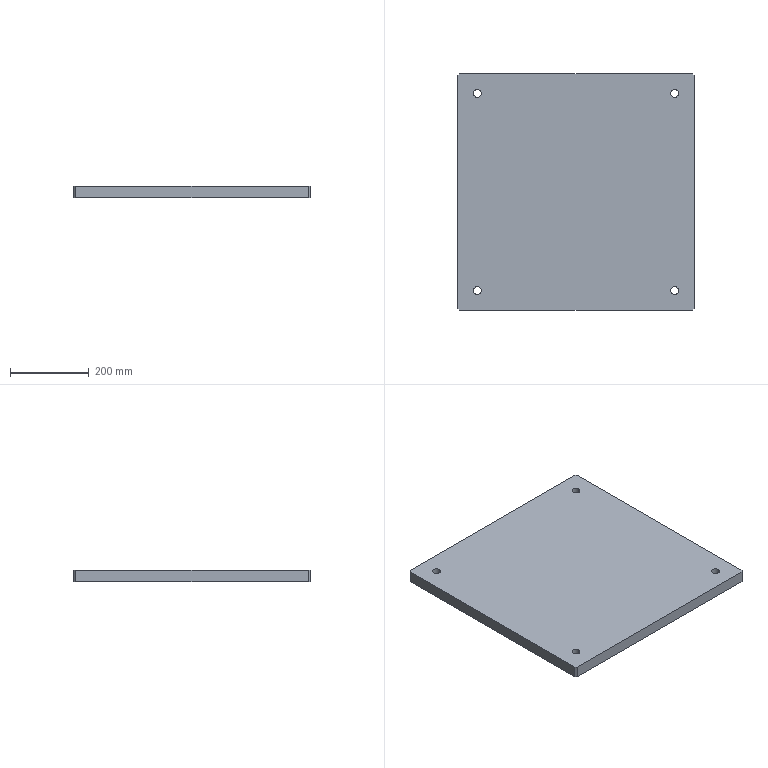Part | NX | features BREP 1 | 1 solid | 18 faces | box 600 x 600 x 30 mm | volume 10760801 mm3 | plane 10 | cylinder 8 | commonest cylinder face diameters 20 x8
STEP:
#1=CARTESIAN_POINT('',(240.,250.,0.));
#2=VERTEX_POINT('',#1);
#3=CARTESIAN_POINT('',(260.,250.,0.));
#4=VERTEX_POINT('',#3);
#5=CARTESIAN_POINT('',(250.,250.,0.));
#6=DIRECTION('',(0.,0.,1.));
#7=DIRECTION('',(1.,0.,0.));
#8=AXIS2_PLACEMENT_3D('',#5,#6,#7);
#9=CIRCLE('',#8,10.);
#10=EDGE_CURVE('',#2,#4,#9,.T.);
#11=ORIENTED_EDGE('',*,*,#10,.F.);
#12=CARTESIAN_POINT('',(240.,250.,30.));
#13=VERTEX_POINT('',#12);
#14=CARTESIAN_POINT('',(240.,250.,0.));
#15=DIRECTION('',(0.,0.,1.));
#16=VECTOR('',#15,1000.);
#17=LINE('',#14,#16);
#18=EDGE_CURVE('',#13,#2,#17,.F.);
#19=ORIENTED_EDGE('',*,*,#18,.F.);
#20=CARTESIAN_POINT('',(260.,250.,30.));
#21=VERTEX_POINT('',#20);
#22=CARTESIAN_POINT('',(250.,250.,30.));
#23=DIRECTION('',(0.,0.,1.));
#24=DIRECTION('',(1.,0.,0.));
#25=AXIS2_PLACEMENT_3D('',#22,#23,#24);
#26=CIRCLE('',#25,10.);
#27=EDGE_CURVE('',#13,#21,#26,.T.);
#28=ORIENTED_EDGE('',*,*,#27,.T.);
#29=CARTESIAN_POINT('',(260.,250.,0.));
#30=DIRECTION('',(0.,0.,1.));
#31=VECTOR('',#30,1000.);
#32=LINE('',#29,#31);
#33=EDGE_CURVE('',#21,#4,#32,.F.);
#34=ORIENTED_EDGE('',*,*,#33,.T.);
#35=EDGE_LOOP('',(#11,#19,#28,#34));
#36=FACE_BOUND('',#35,.T.);
#37=CARTESIAN_POINT('',(250.,250.,0.));
#38=DIRECTION('',(0.,0.,1.));
#39=DIRECTION('',(1.,0.,0.));
#40=AXIS2_PLACEMENT_3D('',#37,#38,#39);
#41=CYLINDRICAL_SURFACE('',#40,10.);
#42=ADVANCED_FACE('',(#36),#41,.F.);
#43=CARTESIAN_POINT('',(-260.,-250.,0.));
#44=VERTEX_POINT('',#43);
#45=CARTESIAN_POINT('',(-240.,-250.,0.));
#46=VERTEX_POINT('',#45);
#47=CARTESIAN_POINT('',(-250.,-250.,0.));
#48=DIRECTION('',(0.,0.,1.));
#49=DIRECTION('',(1.,0.,0.));
#50=AXIS2_PLACEMENT_3D('',#47,#48,#49);
#51=CIRCLE('',#50,10.);
#52=EDGE_CURVE('',#44,#46,#51,.T.);
#53=ORIENTED_EDGE('',*,*,#52,.F.);
#54=CARTESIAN_POINT('',(-260.,-250.,30.));
#55=VERTEX_POINT('',#54);
#56=CARTESIAN_POINT('',(-260.,-250.,0.));
#57=DIRECTION('',(0.,0.,1.));
#58=VECTOR('',#57,1000.);
#59=LINE('',#56,#58);
#60=EDGE_CURVE('',#55,#44,#59,.F.);
#61=ORIENTED_EDGE('',*,*,#60,.F.);
#62=CARTESIAN_POINT('',(-240.,-250.,30.));
#63=VERTEX_POINT('',#62);
#64=CARTESIAN_POINT('',(-250.,-250.,30.));
#65=DIRECTION('',(0.,0.,1.));
#66=DIRECTION('',(1.,0.,0.));
#67=AXIS2_PLACEMENT_3D('',#64,#65,#66);
#68=CIRCLE('',#67,10.);
#69=EDGE_CURVE('',#55,#63,#68,.T.);
#70=ORIENTED_EDGE('',*,*,#69,.T.);
#71=CARTESIAN_POINT('',(-240.,-250.,0.));
#72=DIRECTION('',(0.,0.,1.));
#73=VECTOR('',#72,1000.);
#74=LINE('',#71,#73);
#75=EDGE_CURVE('',#63,#46,#74,.F.);
#76=ORIENTED_EDGE('',*,*,#75,.T.);
#77=EDGE_LOOP('',(#53,#61,#70,#76));
#78=FACE_BOUND('',#77,.T.);
#79=CARTESIAN_POINT('',(-250.,-250.,0.));
#80=DIRECTION('',(0.,0.,1.));
#81=DIRECTION('',(1.,0.,0.));
#82=AXIS2_PLACEMENT_3D('',#79,#80,#81);
#83=CYLINDRICAL_SURFACE('',#82,10.);
#84=ADVANCED_FACE('',(#78),#83,.F.);
#85=CARTESIAN_POINT('',(240.,-250.,0.));
#86=VERTEX_POINT('',#85);
#87=CARTESIAN_POINT('',(260.,-250.,0.));
#88=VERTEX_POINT('',#87);
#89=CARTESIAN_POINT('',(250.,-250.,0.));
#90=DIRECTION('',(0.,0.,1.));
#91=DIRECTION('',(1.,0.,0.));
#92=AXIS2_PLACEMENT_3D('',#89,#90,#91);
#93=CIRCLE('',#92,10.);
#94=EDGE_CURVE('',#86,#88,#93,.T.);
#95=ORIENTED_EDGE('',*,*,#94,.F.);
#96=CARTESIAN_POINT('',(240.,-250.,30.));
#97=VERTEX_POINT('',#96);
#98=CARTESIAN_POINT('',(240.,-250.,0.));
#99=DIRECTION('',(0.,0.,1.));
#100=VECTOR('',#99,1000.);
#101=LINE('',#98,#100);
#102=EDGE_CURVE('',#97,#86,#101,.F.);
#103=ORIENTED_EDGE('',*,*,#102,.F.);
#104=CARTESIAN_POINT('',(260.,-250.,30.));
#105=VERTEX_POINT('',#104);
#106=CARTESIAN_POINT('',(250.,-250.,30.));
#107=DIRECTION('',(0.,0.,1.));
#108=DIRECTION('',(1.,0.,0.));
#109=AXIS2_PLACEMENT_3D('',#106,#107,#108);
#110=CIRCLE('',#109,10.);
#111=EDGE_CURVE('',#97,#105,#110,.T.);
#112=ORIENTED_EDGE('',*,*,#111,.T.);
#113=CARTESIAN_POINT('',(260.,-250.,0.));
#114=DIRECTION('',(0.,0.,1.));
#115=VECTOR('',#114,1000.);
#116=LINE('',#113,#115);
#117=EDGE_CURVE('',#105,#88,#116,.F.);
#118=ORIENTED_EDGE('',*,*,#117,.T.);
#119=EDGE_LOOP('',(#95,#103,#112,#118));
#120=FACE_BOUND('',#119,.T.);
#121=CARTESIAN_POINT('',(250.,-250.,0.));
#122=DIRECTION('',(0.,0.,1.));
#123=DIRECTION('',(1.,0.,0.));
#124=AXIS2_PLACEMENT_3D('',#121,#122,#123);
#125=CYLINDRICAL_SURFACE('',#124,10.);
#126=ADVANCED_FACE('',(#120),#125,.F.);
#127=CARTESIAN_POINT('',(-260.,250.,0.));
#128=VERTEX_POINT('',#127);
#129=CARTESIAN_POINT('',(-240.,250.,0.));
#130=VERTEX_POINT('',#129);
#131=CARTESIAN_POINT('',(-250.,250.,0.));
#132=DIRECTION('',(0.,0.,1.));
#133=DIRECTION('',(1.,0.,0.));
#134=AXIS2_PLACEMENT_3D('',#131,#132,#133);
#135=CIRCLE('',#134,10.);
#136=EDGE_CURVE('',#128,#130,#135,.T.);
#137=ORIENTED_EDGE('',*,*,#136,.F.);
#138=CARTESIAN_POINT('',(-260.,250.,30.));
#139=VERTEX_POINT('',#138);
#140=CARTESIAN_POINT('',(-260.,250.,0.));
#141=DIRECTION('',(0.,0.,1.));
#142=VECTOR('',#141,1000.);
#143=LINE('',#140,#142);
#144=EDGE_CURVE('',#139,#128,#143,.F.);
#145=ORIENTED_EDGE('',*,*,#144,.F.);
#146=CARTESIAN_POINT('',(-240.,250.,30.));
#147=VERTEX_POINT('',#146);
#148=CARTESIAN_POINT('',(-250.,250.,30.));
#149=DIRECTION('',(0.,0.,1.));
#150=DIRECTION('',(1.,0.,0.));
#151=AXIS2_PLACEMENT_3D('',#148,#149,#150);
#152=CIRCLE('',#151,10.);
#153=EDGE_CURVE('',#139,#147,#152,.T.);
#154=ORIENTED_EDGE('',*,*,#153,.T.);
#155=CARTESIAN_POINT('',(-240.,250.,0.));
#156=DIRECTION('',(0.,0.,1.));
#157=VECTOR('',#156,1000.);
#158=LINE('',#155,#157);
#159=EDGE_CURVE('',#147,#130,#158,.F.);
#160=ORIENTED_EDGE('',*,*,#159,.T.);
#161=EDGE_LOOP('',(#137,#145,#154,#160));
#162=FACE_BOUND('',#161,.T.);
#163=CARTESIAN_POINT('',(-250.,250.,0.));
#164=DIRECTION('',(0.,0.,1.));
#165=DIRECTION('',(1.,0.,0.));
#166=AXIS2_PLACEMENT_3D('',#163,#164,#165);
#167=CYLINDRICAL_SURFACE('',#166,10.);
#168=ADVANCED_FACE('',(#162),#167,.F.);
#169=CARTESIAN_POINT('',(300.,-295.,0.));
#170=VERTEX_POINT('',#169);
#171=CARTESIAN_POINT('',(300.,295.,0.));
#172=VERTEX_POINT('',#171);
#173=CARTESIAN_POINT('',(300.,300.,0.));
#174=DIRECTION('',(0.,1.,0.));
#175=VECTOR('',#174,1000.);
#176=LINE('',#173,#175);
#177=EDGE_CURVE('',#170,#172,#176,.T.);
#178=ORIENTED_EDGE('',*,*,#177,.T.);
#179=CARTESIAN_POINT('',(300.,295.,30.));
#180=VERTEX_POINT('',#179);
#181=CARTESIAN_POINT('',(300.,295.,30.));
#182=DIRECTION('',(0.,0.,1.));
#183=VECTOR('',#182,1000.);
#184=LINE('',#181,#183);
#185=EDGE_CURVE('',#172,#180,#184,.T.);
#186=ORIENTED_EDGE('',*,*,#185,.T.);
#187=CARTESIAN_POINT('',(300.,-295.,30.));
#188=VERTEX_POINT('',#187);
#189=CARTESIAN_POINT('',(300.,300.,30.));
#190=DIRECTION('',(0.,1.,0.));
#191=VECTOR('',#190,1000.);
#192=LINE('',#189,#191);
#193=EDGE_CURVE('',#188,#180,#192,.T.);
#194=ORIENTED_EDGE('',*,*,#193,.F.);
#195=CARTESIAN_POINT('',(300.,-295.,30.));
#196=DIRECTION('',(0.,0.,-1.));
#197=VECTOR('',#196,1000.);
#198=LINE('',#195,#197);
#199=EDGE_CURVE('',#188,#170,#198,.T.);
#200=ORIENTED_EDGE('',*,*,#199,.T.);
#201=EDGE_LOOP('',(#178,#186,#194,#200));
#202=FACE_BOUND('',#201,.T.);
#203=CARTESIAN_POINT('',(300.,300.,30.));
#204=DIRECTION('',(-1.,0.,0.));
#205=DIRECTION('',(0.,1.,0.));
#206=AXIS2_PLACEMENT_3D('',#203,#204,#205);
#207=PLANE('',#206);
#208=ADVANCED_FACE('',(#202),#207,.F.);
#209=CARTESIAN_POINT('',(295.,300.,30.));
#210=VERTEX_POINT('',#209);
#211=CARTESIAN_POINT('',(-295.,300.,30.));
#212=VERTEX_POINT('',#211);
#213=CARTESIAN_POINT('',(-300.,300.,30.));
#214=DIRECTION('',(-1.,0.,0.));
#215=VECTOR('',#214,1000.);
#216=LINE('',#213,#215);
#217=EDGE_CURVE('',#210,#212,#216,.T.);
#218=ORIENTED_EDGE('',*,*,#217,.F.);
#219=CARTESIAN_POINT('',(295.,300.,0.));
#220=VERTEX_POINT('',#219);
#221=CARTESIAN_POINT('',(295.,300.,30.));
#222=DIRECTION('',(0.,0.,-1.));
#223=VECTOR('',#222,1000.);
#224=LINE('',#221,#223);
#225=EDGE_CURVE('',#210,#220,#224,.T.);
#226=ORIENTED_EDGE('',*,*,#225,.T.);
#227=CARTESIAN_POINT('',(-295.,300.,0.));
#228=VERTEX_POINT('',#227);
#229=CARTESIAN_POINT('',(-300.,300.,0.));
#230=DIRECTION('',(-1.,0.,0.));
#231=VECTOR('',#230,1000.);
#232=LINE('',#229,#231);
#233=EDGE_CURVE('',#220,#228,#232,.T.);
#234=ORIENTED_EDGE('',*,*,#233,.T.);
#235=CARTESIAN_POINT('',(-295.,300.,30.));
#236=DIRECTION('',(0.,0.,1.));
#237=VECTOR('',#236,1000.);
#238=LINE('',#235,#237);
#239=EDGE_CURVE('',#228,#212,#238,.T.);
#240=ORIENTED_EDGE('',*,*,#239,.T.);
#241=EDGE_LOOP('',(#218,#226,#234,#240));
#242=FACE_BOUND('',#241,.T.);
#243=CARTESIAN_POINT('',(-300.,300.,30.));
#244=DIRECTION('',(0.,-1.,0.));
#245=DIRECTION('',(0.,0.,-1.));
#246=AXIS2_PLACEMENT_3D('',#243,#244,#245);
#247=PLANE('',#246);
#248=ADVANCED_FACE('',(#242),#247,.F.);
#249=CARTESIAN_POINT('',(-300.,295.,0.));
#250=VERTEX_POINT('',#249);
#251=CARTESIAN_POINT('',(-300.,-295.,0.));
#252=VERTEX_POINT('',#251);
#253=CARTESIAN_POINT('',(-300.,300.,0.));
#254=DIRECTION('',(0.,-1.,0.));
#255=VECTOR('',#254,1000.);
#256=LINE('',#253,#255);
#257=EDGE_CURVE('',#250,#252,#256,.T.);
#258=ORIENTED_EDGE('',*,*,#257,.T.);
#259=CARTESIAN_POINT('',(-300.,-295.,30.));
#260=VERTEX_POINT('',#259);
#261=CARTESIAN_POINT('',(-300.,-295.,30.));
#262=DIRECTION('',(0.,0.,1.));
#263=VECTOR('',#262,1000.);
#264=LINE('',#261,#263);
#265=EDGE_CURVE('',#252,#260,#264,.T.);
#266=ORIENTED_EDGE('',*,*,#265,.T.);
#267=CARTESIAN_POINT('',(-300.,295.,30.));
#268=VERTEX_POINT('',#267);
#269=CARTESIAN_POINT('',(-300.,300.,30.));
#270=DIRECTION('',(0.,-1.,0.));
#271=VECTOR('',#270,1000.);
#272=LINE('',#269,#271);
#273=EDGE_CURVE('',#268,#260,#272,.T.);
#274=ORIENTED_EDGE('',*,*,#273,.F.);
#275=CARTESIAN_POINT('',(-300.,295.,30.));
#276=DIRECTION('',(0.,0.,-1.));
#277=VECTOR('',#276,1000.);
#278=LINE('',#275,#277);
#279=EDGE_CURVE('',#268,#250,#278,.T.);
#280=ORIENTED_EDGE('',*,*,#279,.T.);
#281=EDGE_LOOP('',(#258,#266,#274,#280));
#282=FACE_BOUND('',#281,.T.);
#283=CARTESIAN_POINT('',(-300.,300.,30.));
#284=DIRECTION('',(1.,0.,0.));
#285=DIRECTION('',(0.,1.,0.));
#286=AXIS2_PLACEMENT_3D('',#283,#284,#285);
#287=PLANE('',#286);
#288=ADVANCED_FACE('',(#282),#287,.F.);
#289=CARTESIAN_POINT('',(-295.,-300.,0.));
#290=VERTEX_POINT('',#289);
#291=CARTESIAN_POINT('',(295.,-300.,0.));
#292=VERTEX_POINT('',#291);
#293=CARTESIAN_POINT('',(-300.,-300.,0.));
#294=DIRECTION('',(1.,0.,0.));
#295=VECTOR('',#294,1000.);
#296=LINE('',#293,#295);
#297=EDGE_CURVE('',#290,#292,#296,.T.);
#298=ORIENTED_EDGE('',*,*,#297,.T.);
#299=CARTESIAN_POINT('',(295.,-300.,30.));
#300=VERTEX_POINT('',#299);
#301=CARTESIAN_POINT('',(295.,-300.,30.));
#302=DIRECTION('',(0.,0.,1.));
#303=VECTOR('',#302,1000.);
#304=LINE('',#301,#303);
#305=EDGE_CURVE('',#292,#300,#304,.T.);
#306=ORIENTED_EDGE('',*,*,#305,.T.);
#307=CARTESIAN_POINT('',(-295.,-300.,30.));
#308=VERTEX_POINT('',#307);
#309=CARTESIAN_POINT('',(-300.,-300.,30.));
#310=DIRECTION('',(1.,0.,0.));
#311=VECTOR('',#310,1000.);
#312=LINE('',#309,#311);
#313=EDGE_CURVE('',#308,#300,#312,.T.);
#314=ORIENTED_EDGE('',*,*,#313,.F.);
#315=CARTESIAN_POINT('',(-295.,-300.,30.));
#316=DIRECTION('',(0.,0.,-1.));
#317=VECTOR('',#316,1000.);
#318=LINE('',#315,#317);
#319=EDGE_CURVE('',#308,#290,#318,.T.);
#320=ORIENTED_EDGE('',*,*,#319,.T.);
#321=EDGE_LOOP('',(#298,#306,#314,#320));
#322=FACE_BOUND('',#321,.T.);
#323=CARTESIAN_POINT('',(-300.,-300.,30.));
#324=DIRECTION('',(0.,1.,0.));
#325=DIRECTION('',(1.,0.,0.));
#326=AXIS2_PLACEMENT_3D('',#323,#324,#325);
#327=PLANE('',#326);
#328=ADVANCED_FACE('',(#322),#327,.F.);
#329=ORIENTED_EDGE('',*,*,#193,.T.);
#330=CARTESIAN_POINT('',(297.5,297.5,30.));
#331=DIRECTION('',(-0.7071,0.7071,0.));
#332=VECTOR('',#331,1000.);
#333=LINE('',#330,#332);
#334=EDGE_CURVE('',#180,#210,#333,.T.);
#335=ORIENTED_EDGE('',*,*,#334,.T.);
#336=ORIENTED_EDGE('',*,*,#217,.T.);
#337=CARTESIAN_POINT('',(-297.5,297.5,30.));
#338=DIRECTION('',(-0.7071,-0.7071,0.));
#339=VECTOR('',#338,1000.);
#340=LINE('',#337,#339);
#341=EDGE_CURVE('',#212,#268,#340,.T.);
#342=ORIENTED_EDGE('',*,*,#341,.T.);
#343=ORIENTED_EDGE('',*,*,#273,.T.);
#344=CARTESIAN_POINT('',(-297.5,-297.5,30.));
#345=DIRECTION('',(0.7071,-0.7071,0.));
#346=VECTOR('',#345,1000.);
#347=LINE('',#344,#346);
#348=EDGE_CURVE('',#260,#308,#347,.T.);
#349=ORIENTED_EDGE('',*,*,#348,.T.);
#350=ORIENTED_EDGE('',*,*,#313,.T.);
#351=CARTESIAN_POINT('',(297.5,-297.5,30.));
#352=DIRECTION('',(0.7071,0.7071,0.));
#353=VECTOR('',#352,1000.);
#354=LINE('',#351,#353);
#355=EDGE_CURVE('',#300,#188,#354,.T.);
#356=ORIENTED_EDGE('',*,*,#355,.T.);
#357=EDGE_LOOP('',(#329,#335,#336,#342,#343,#349,#350,#356));
#358=FACE_BOUND('',#357,.T.);
#359=CARTESIAN_POINT('',(250.,250.,30.));
#360=DIRECTION('',(0.,0.,1.));
#361=DIRECTION('',(1.,0.,0.));
#362=AXIS2_PLACEMENT_3D('',#359,#360,#361);
#363=CIRCLE('',#362,10.);
#364=EDGE_CURVE('',#21,#13,#363,.T.);
#365=ORIENTED_EDGE('',*,*,#364,.F.);
#366=ORIENTED_EDGE('',*,*,#27,.F.);
#367=EDGE_LOOP('',(#365,#366));
#368=FACE_BOUND('',#367,.T.);
#369=CARTESIAN_POINT('',(-250.,-250.,30.));
#370=DIRECTION('',(0.,0.,1.));
#371=DIRECTION('',(1.,0.,0.));
#372=AXIS2_PLACEMENT_3D('',#369,#370,#371);
#373=CIRCLE('',#372,10.);
#374=EDGE_CURVE('',#63,#55,#373,.T.);
#375=ORIENTED_EDGE('',*,*,#374,.F.);
#376=ORIENTED_EDGE('',*,*,#69,.F.);
#377=EDGE_LOOP('',(#375,#376));
#378=FACE_BOUND('',#377,.T.);
#379=CARTESIAN_POINT('',(250.,-250.,30.));
#380=DIRECTION('',(0.,0.,1.));
#381=DIRECTION('',(1.,0.,0.));
#382=AXIS2_PLACEMENT_3D('',#379,#380,#381);
#383=CIRCLE('',#382,10.);
#384=EDGE_CURVE('',#105,#97,#383,.T.);
#385=ORIENTED_EDGE('',*,*,#384,.F.);
#386=ORIENTED_EDGE('',*,*,#111,.F.);
#387=EDGE_LOOP('',(#385,#386));
#388=FACE_BOUND('',#387,.T.);
#389=CARTESIAN_POINT('',(-250.,250.,30.));
#390=DIRECTION('',(0.,0.,1.));
#391=DIRECTION('',(1.,0.,0.));
#392=AXIS2_PLACEMENT_3D('',#389,#390,#391);
#393=CIRCLE('',#392,10.);
#394=EDGE_CURVE('',#147,#139,#393,.T.);
#395=ORIENTED_EDGE('',*,*,#394,.F.);
#396=ORIENTED_EDGE('',*,*,#153,.F.);
#397=EDGE_LOOP('',(#395,#396));
#398=FACE_BOUND('',#397,.T.);
#399=CARTESIAN_POINT('',(0.,0.,30.));
#400=DIRECTION('',(0.,0.,1.));
#401=DIRECTION('',(1.,0.,0.));
#402=AXIS2_PLACEMENT_3D('',#399,#400,#401);
#403=PLANE('',#402);
#404=ADVANCED_FACE('',(#358,#368,#378,#388,#398),#403,.T.);
#405=ORIENTED_EDGE('',*,*,#233,.F.);
#406=CARTESIAN_POINT('',(295.,300.,0.));
#407=DIRECTION('',(0.7071,-0.7071,0.));
#408=VECTOR('',#407,1000.);
#409=LINE('',#406,#408);
#410=EDGE_CURVE('',#220,#172,#409,.T.);
#411=ORIENTED_EDGE('',*,*,#410,.T.);
#412=ORIENTED_EDGE('',*,*,#177,.F.);
#413=CARTESIAN_POINT('',(300.,-295.,0.));
#414=DIRECTION('',(-0.7071,-0.7071,0.));
#415=VECTOR('',#414,1000.);
#416=LINE('',#413,#415);
#417=EDGE_CURVE('',#170,#292,#416,.T.);
#418=ORIENTED_EDGE('',*,*,#417,.T.);
#419=ORIENTED_EDGE('',*,*,#297,.F.);
#420=CARTESIAN_POINT('',(-295.,-300.,0.));
#421=DIRECTION('',(-0.7071,0.7071,0.));
#422=VECTOR('',#421,1000.);
#423=LINE('',#420,#422);
#424=EDGE_CURVE('',#290,#252,#423,.T.);
#425=ORIENTED_EDGE('',*,*,#424,.T.);
#426=ORIENTED_EDGE('',*,*,#257,.F.);
#427=CARTESIAN_POINT('',(-300.,295.,0.));
#428=DIRECTION('',(0.7071,0.7071,0.));
#429=VECTOR('',#428,1000.);
#430=LINE('',#427,#429);
#431=EDGE_CURVE('',#250,#228,#430,.T.);
#432=ORIENTED_EDGE('',*,*,#431,.T.);
#433=EDGE_LOOP('',(#405,#411,#412,#418,#419,#425,#426,#432));
#434=FACE_BOUND('',#433,.T.);
#435=CARTESIAN_POINT('',(250.,250.,0.));
#436=DIRECTION('',(0.,0.,1.));
#437=DIRECTION('',(1.,0.,0.));
#438=AXIS2_PLACEMENT_3D('',#435,#436,#437);
#439=CIRCLE('',#438,10.);
#440=EDGE_CURVE('',#4,#2,#439,.T.);
#441=ORIENTED_EDGE('',*,*,#440,.T.);
#442=ORIENTED_EDGE('',*,*,#10,.T.);
#443=EDGE_LOOP('',(#441,#442));
#444=FACE_BOUND('',#443,.T.);
#445=CARTESIAN_POINT('',(-250.,-250.,0.));
#446=DIRECTION('',(0.,0.,1.));
#447=DIRECTION('',(1.,0.,0.));
#448=AXIS2_PLACEMENT_3D('',#445,#446,#447);
#449=CIRCLE('',#448,10.);
#450=EDGE_CURVE('',#46,#44,#449,.T.);
#451=ORIENTED_EDGE('',*,*,#450,.T.);
#452=ORIENTED_EDGE('',*,*,#52,.T.);
#453=EDGE_LOOP('',(#451,#452));
#454=FACE_BOUND('',#453,.T.);
#455=CARTESIAN_POINT('',(250.,-250.,0.));
#456=DIRECTION('',(0.,0.,1.));
#457=DIRECTION('',(1.,0.,0.));
#458=AXIS2_PLACEMENT_3D('',#455,#456,#457);
#459=CIRCLE('',#458,10.);
#460=EDGE_CURVE('',#88,#86,#459,.T.);
#461=ORIENTED_EDGE('',*,*,#460,.T.);
#462=ORIENTED_EDGE('',*,*,#94,.T.);
#463=EDGE_LOOP('',(#461,#462));
#464=FACE_BOUND('',#463,.T.);
#465=CARTESIAN_POINT('',(-250.,250.,0.));
#466=DIRECTION('',(0.,0.,1.));
#467=DIRECTION('',(1.,0.,0.));
#468=AXIS2_PLACEMENT_3D('',#465,#466,#467);
#469=CIRCLE('',#468,10.);
#470=EDGE_CURVE('',#130,#128,#469,.T.);
#471=ORIENTED_EDGE('',*,*,#470,.T.);
#472=ORIENTED_EDGE('',*,*,#136,.T.);
#473=EDGE_LOOP('',(#471,#472));
#474=FACE_BOUND('',#473,.T.);
#475=CARTESIAN_POINT('',(0.,0.,0.));
#476=DIRECTION('',(0.,0.,1.));
#477=DIRECTION('',(1.,0.,0.));
#478=AXIS2_PLACEMENT_3D('',#475,#476,#477);
#479=PLANE('',#478);
#480=ADVANCED_FACE('',(#434,#444,#454,#464,#474),#479,.F.);
#481=ORIENTED_EDGE('',*,*,#334,.F.);
#482=ORIENTED_EDGE('',*,*,#185,.F.);
#483=ORIENTED_EDGE('',*,*,#410,.F.);
#484=ORIENTED_EDGE('',*,*,#225,.F.);
#485=EDGE_LOOP('',(#481,#482,#483,#484));
#486=FACE_BOUND('',#485,.T.);
#487=CARTESIAN_POINT('',(295.,300.,30.));
#488=DIRECTION('',(-0.7071,-0.7071,0.));
#489=DIRECTION('',(-0.7071,0.7071,0.));
#490=AXIS2_PLACEMENT_3D('',#487,#488,#489);
#491=PLANE('',#490);
#492=ADVANCED_FACE('',(#486),#491,.F.);
#493=ORIENTED_EDGE('',*,*,#355,.F.);
#494=ORIENTED_EDGE('',*,*,#305,.F.);
#495=ORIENTED_EDGE('',*,*,#417,.F.);
#496=ORIENTED_EDGE('',*,*,#199,.F.);
#497=EDGE_LOOP('',(#493,#494,#495,#496));
#498=FACE_BOUND('',#497,.T.);
#499=CARTESIAN_POINT('',(300.,-295.,30.));
#500=DIRECTION('',(-0.7071,0.7071,0.));
#501=DIRECTION('',(0.,0.,1.));
#502=AXIS2_PLACEMENT_3D('',#499,#500,#501);
#503=PLANE('',#502);
#504=ADVANCED_FACE('',(#498),#503,.F.);
#505=ORIENTED_EDGE('',*,*,#348,.F.);
#506=ORIENTED_EDGE('',*,*,#265,.F.);
#507=ORIENTED_EDGE('',*,*,#424,.F.);
#508=ORIENTED_EDGE('',*,*,#319,.F.);
#509=EDGE_LOOP('',(#505,#506,#507,#508));
#510=FACE_BOUND('',#509,.T.);
#511=CARTESIAN_POINT('',(-295.,-300.,30.));
#512=DIRECTION('',(0.7071,0.7071,0.));
#513=DIRECTION('',(0.,0.,-1.));
#514=AXIS2_PLACEMENT_3D('',#511,#512,#513);
#515=PLANE('',#514);
#516=ADVANCED_FACE('',(#510),#515,.F.);
#517=ORIENTED_EDGE('',*,*,#341,.F.);
#518=ORIENTED_EDGE('',*,*,#239,.F.);
#519=ORIENTED_EDGE('',*,*,#431,.F.);
#520=ORIENTED_EDGE('',*,*,#279,.F.);
#521=EDGE_LOOP('',(#517,#518,#519,#520));
#522=FACE_BOUND('',#521,.T.);
#523=CARTESIAN_POINT('',(-300.,295.,30.));
#524=DIRECTION('',(0.7071,-0.7071,0.));
#525=DIRECTION('',(0.,0.,-1.));
#526=AXIS2_PLACEMENT_3D('',#523,#524,#525);
#527=PLANE('',#526);
#528=ADVANCED_FACE('',(#522),#527,.F.);
#529=ORIENTED_EDGE('',*,*,#144,.T.);
#530=ORIENTED_EDGE('',*,*,#470,.F.);
#531=ORIENTED_EDGE('',*,*,#159,.F.);
#532=ORIENTED_EDGE('',*,*,#394,.T.);
#533=EDGE_LOOP('',(#529,#530,#531,#532));
#534=FACE_BOUND('',#533,.T.);
#535=CARTESIAN_POINT('',(-250.,250.,0.));
#536=DIRECTION('',(0.,0.,1.));
#537=DIRECTION('',(1.,0.,0.));
#538=AXIS2_PLACEMENT_3D('',#535,#536,#537);
#539=CYLINDRICAL_SURFACE('',#538,10.);
#540=ADVANCED_FACE('',(#534),#539,.F.);
#541=ORIENTED_EDGE('',*,*,#102,.T.);
#542=ORIENTED_EDGE('',*,*,#460,.F.);
#543=ORIENTED_EDGE('',*,*,#117,.F.);
#544=ORIENTED_EDGE('',*,*,#384,.T.);
#545=EDGE_LOOP('',(#541,#542,#543,#544));
#546=FACE_BOUND('',#545,.T.);
#547=CARTESIAN_POINT('',(250.,-250.,0.));
#548=DIRECTION('',(0.,0.,1.));
#549=DIRECTION('',(1.,0.,0.));
#550=AXIS2_PLACEMENT_3D('',#547,#548,#549);
#551=CYLINDRICAL_SURFACE('',#550,10.);
#552=ADVANCED_FACE('',(#546),#551,.F.);
#553=ORIENTED_EDGE('',*,*,#60,.T.);
#554=ORIENTED_EDGE('',*,*,#450,.F.);
#555=ORIENTED_EDGE('',*,*,#75,.F.);
#556=ORIENTED_EDGE('',*,*,#374,.T.);
#557=EDGE_LOOP('',(#553,#554,#555,#556));
#558=FACE_BOUND('',#557,.T.);
#559=CARTESIAN_POINT('',(-250.,-250.,0.));
#560=DIRECTION('',(0.,0.,1.));
#561=DIRECTION('',(1.,0.,0.));
#562=AXIS2_PLACEMENT_3D('',#559,#560,#561);
#563=CYLINDRICAL_SURFACE('',#562,10.);
#564=ADVANCED_FACE('',(#558),#563,.F.);
#565=ORIENTED_EDGE('',*,*,#18,.T.);
#566=ORIENTED_EDGE('',*,*,#440,.F.);
#567=ORIENTED_EDGE('',*,*,#33,.F.);
#568=ORIENTED_EDGE('',*,*,#364,.T.);
#569=EDGE_LOOP('',(#565,#566,#567,#568));
#570=FACE_BOUND('',#569,.T.);
#571=CARTESIAN_POINT('',(250.,250.,0.));
#572=DIRECTION('',(0.,0.,1.));
#573=DIRECTION('',(1.,0.,0.));
#574=AXIS2_PLACEMENT_3D('',#571,#572,#573);
#575=CYLINDRICAL_SURFACE('',#574,10.);
#576=ADVANCED_FACE('',(#570),#575,.F.);
#577=CLOSED_SHELL('',(#42,#84,#126,#168,#208,#248,#288,#328,#404,#480,#492,#504,#516,#528,#540,#552,#564,#576));
#578=MANIFOLD_SOLID_BREP('',#577);
#579=(LENGTH_UNIT()NAMED_UNIT(*)SI_UNIT(.MILLI.,.METRE.));
#580=UNCERTAINTY_MEASURE_WITH_UNIT(LENGTH_MEASURE(0.00001),#579,'','');
#581=(NAMED_UNIT(*)PLANE_ANGLE_UNIT()SI_UNIT($,.RADIAN.));
#582=(NAMED_UNIT(*)SI_UNIT($,.STERADIAN.)SOLID_ANGLE_UNIT());
#583=(GEOMETRIC_REPRESENTATION_CONTEXT(3)GLOBAL_UNCERTAINTY_ASSIGNED_CONTEXT((#580))GLOBAL_UNIT_ASSIGNED_CONTEXT((#579,#581,#582))REPRESENTATION_CONTEXT('',''));
#584=ADVANCED_BREP_SHAPE_REPRESENTATION('',(#578),#583);